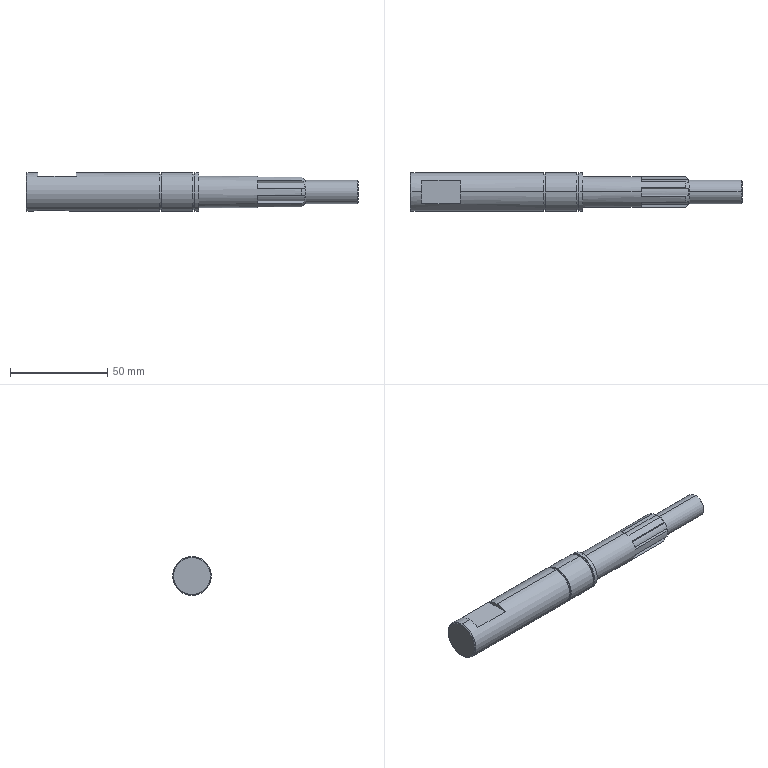Part | SolidWorks | features ICE 9, Chamfer 2, Extrusion 1 | 1 solid | 61 faces | box 171 x 20 x 20 mm | volume 40308 mm3 | plane 31 | cylinder 24 | cone 6 | commonest cylinder face diameters 13 x7 20 x6 18.5 x4 6 x3 12 x2 16 x2